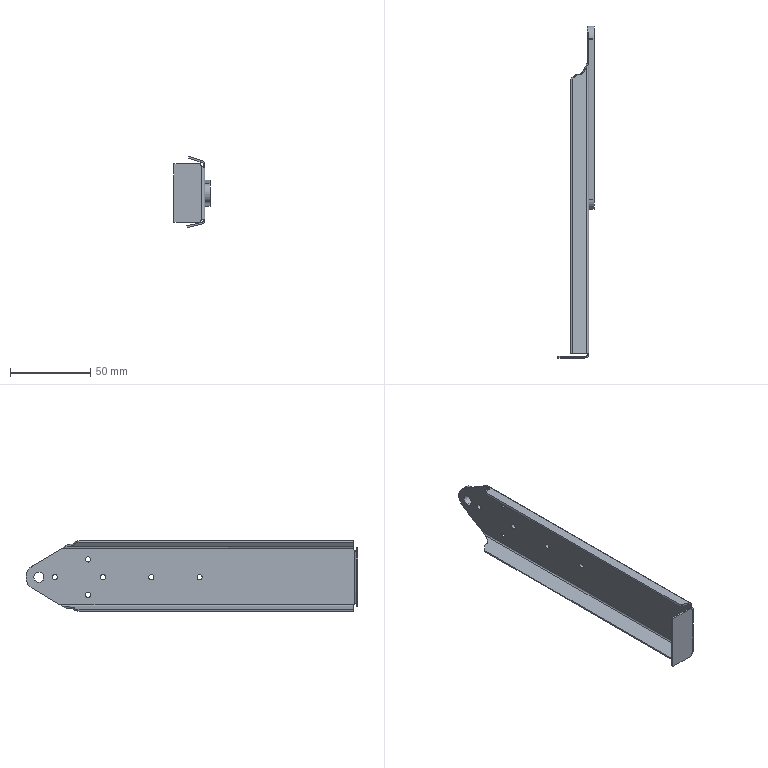Part | SolidWorks | features BaseBody 1 | 1 solid | 62 faces | box 22.422 x 206.522 x 44.137 mm | volume 16299 mm3 | cylinder 30 | plane 26 | spline 6 | commonest cylinder face diameters 3.2 x12 4 x7 2 x3 16 x3 5 x2 6.35 x2